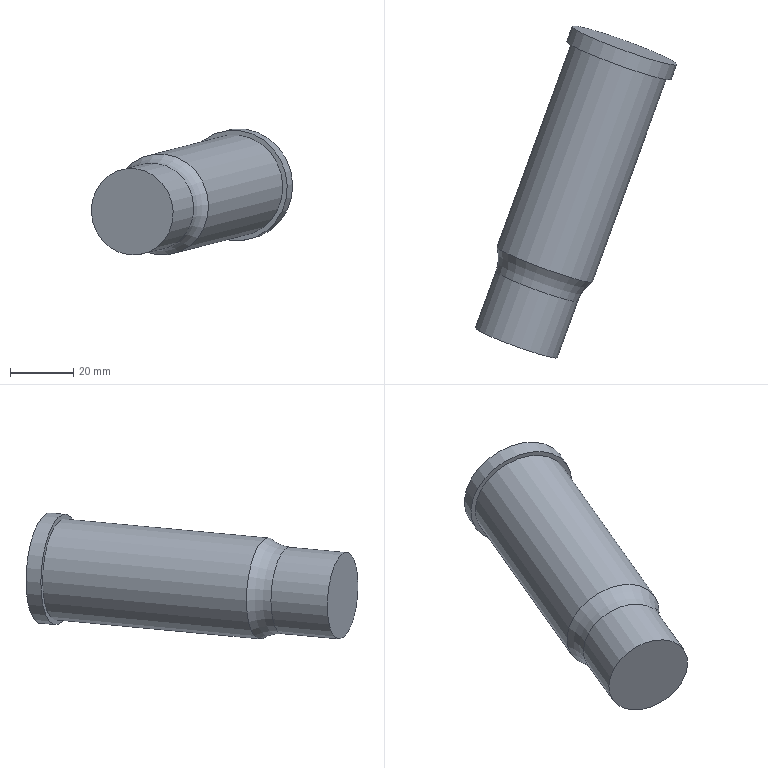Part | NX | features solid 2 | 1 solid | 7 faces | box 63.414 x 104.588 x 39.807 mm | volume 76067 mm3 | cylinder 3 | plane 3 | torus 1 | commonest cylinder face diameters 27.42 x1 32 x1 35 x1
STEP:
#1=CARTESIAN_POINT('',(-630.428,136.085,-11.472));
#2=VERTEX_POINT('',#1);
#3=CARTESIAN_POINT('',(-646.873,142.071,-11.472));
#4=DIRECTION('',(-0.3407,-0.9361,-0.08716));
#5=DIRECTION('',(0.9397,-0.342,0.));
#6=AXIS2_PLACEMENT_3D('',#3,#4,#5);
#7=CIRCLE('',#6,17.5);
#8=EDGE_CURVE('',#2,#2,#7,.T.);
#9=ORIENTED_EDGE('',*,*,#8,.F.);
#10=EDGE_LOOP('',(#9));
#11=FACE_BOUND('',#10,.T.);
#12=CARTESIAN_POINT('',(-628.725,140.766,-11.037));
#13=VERTEX_POINT('',#12);
#14=CARTESIAN_POINT('',(-645.169,146.751,-11.037));
#15=DIRECTION('',(-0.3407,-0.9361,-0.08716));
#16=DIRECTION('',(0.9397,-0.342,0.));
#17=AXIS2_PLACEMENT_3D('',#14,#15,#16);
#18=CIRCLE('',#17,17.5);
#19=EDGE_CURVE('',#13,#13,#18,.T.);
#20=ORIENTED_EDGE('',*,*,#19,.T.);
#21=EDGE_LOOP('',(#20));
#22=FACE_BOUND('',#21,.T.);
#23=CARTESIAN_POINT('',(-653.687,123.348,-13.216));
#24=DIRECTION('',(0.3407,0.9361,0.08716));
#25=DIRECTION('',(-0.9397,0.342,0.));
#26=AXIS2_PLACEMENT_3D('',#23,#24,#25);
#27=CYLINDRICAL_SURFACE('',#26,17.5);
#28=ADVANCED_FACE('',(#11,#22),#27,.T.);
#29=CARTESIAN_POINT('',(-631.838,136.598,-11.472));
#30=VERTEX_POINT('',#29);
#31=CARTESIAN_POINT('',(-646.873,142.071,-11.472));
#32=DIRECTION('',(-0.3407,-0.9361,-0.08716));
#33=DIRECTION('',(0.9397,-0.342,0.));
#34=AXIS2_PLACEMENT_3D('',#31,#32,#33);
#35=CIRCLE('',#34,16.);
#36=EDGE_CURVE('',#30,#30,#35,.T.);
#37=ORIENTED_EDGE('',*,*,#36,.F.);
#38=EDGE_LOOP('',(#37));
#39=FACE_BOUND('',#38,.T.);
#40=ORIENTED_EDGE('',*,*,#8,.T.);
#41=EDGE_LOOP('',(#40));
#42=FACE_BOUND('',#41,.T.);
#43=CARTESIAN_POINT('',(-646.873,142.071,-11.472));
#44=DIRECTION('',(-0.3407,-0.9361,-0.08716));
#45=DIRECTION('',(0.9397,-0.342,0.));
#46=AXIS2_PLACEMENT_3D('',#43,#44,#45);
#47=PLANE('',#46);
#48=ADVANCED_FACE('',(#39,#42),#47,.T.);
#49=ORIENTED_EDGE('',*,*,#19,.F.);
#50=EDGE_LOOP('',(#49));
#51=FACE_BOUND('',#50,.T.);
#52=CARTESIAN_POINT('',(-645.169,146.751,-11.037));
#53=DIRECTION('',(-0.3407,-0.9361,-0.08716));
#54=DIRECTION('',(0.9397,-0.342,0.));
#55=AXIS2_PLACEMENT_3D('',#52,#53,#54);
#56=PLANE('',#55);
#57=ADVANCED_FACE('',(#51),#56,.F.);
#58=ORIENTED_EDGE('',*,*,#36,.T.);
#59=EDGE_LOOP('',(#58));
#60=FACE_BOUND('',#59,.T.);
#61=CARTESIAN_POINT('',(-655.222,72.351,-17.454));
#62=VERTEX_POINT('',#61);
#63=CARTESIAN_POINT('',(-670.257,77.824,-17.454));
#64=DIRECTION('',(-0.3407,-0.9361,-0.08716));
#65=DIRECTION('',(0.9397,-0.342,0.));
#66=AXIS2_PLACEMENT_3D('',#63,#64,#65);
#67=CIRCLE('',#66,16.);
#68=EDGE_CURVE('',#62,#62,#67,.T.);
#69=ORIENTED_EDGE('',*,*,#68,.F.);
#70=EDGE_LOOP('',(#69));
#71=FACE_BOUND('',#70,.T.);
#72=CARTESIAN_POINT('',(-653.687,123.348,-13.216));
#73=DIRECTION('',(-0.3407,-0.9361,-0.08716));
#74=DIRECTION('',(0.9397,-0.342,0.));
#75=AXIS2_PLACEMENT_3D('',#72,#73,#74);
#76=CYLINDRICAL_SURFACE('',#75,16.);
#77=ADVANCED_FACE('',(#60,#71),#76,.T.);
#78=CARTESIAN_POINT('',(-685.651,75.615,-18.096));
#79=VERTEX_POINT('',#78);
#80=CARTESIAN_POINT('',(-672.767,70.926,-18.096));
#81=DIRECTION('',(0.3407,0.9361,0.08716));
#82=DIRECTION('',(-0.9397,0.342,0.));
#83=AXIS2_PLACEMENT_3D('',#80,#81,#82);
#84=CIRCLE('',#83,13.71);
#85=EDGE_CURVE('',#79,#79,#84,.F.);
#86=ORIENTED_EDGE('',*,*,#85,.T.);
#87=EDGE_LOOP('',(#86));
#88=FACE_BOUND('',#87,.T.);
#89=CARTESIAN_POINT('',(-666.358,48.451,-19.752));
#90=VERTEX_POINT('',#89);
#91=CARTESIAN_POINT('',(-679.241,53.14,-19.752));
#92=DIRECTION('',(-0.3407,-0.9361,-0.08716));
#93=DIRECTION('',(0.9397,-0.342,0.));
#94=AXIS2_PLACEMENT_3D('',#91,#92,#93);
#95=CIRCLE('',#94,13.71);
#96=EDGE_CURVE('',#90,#90,#95,.T.);
#97=ORIENTED_EDGE('',*,*,#96,.F.);
#98=EDGE_LOOP('',(#97));
#99=FACE_BOUND('',#98,.T.);
#100=CARTESIAN_POINT('',(-679.241,53.14,-19.752));
#101=DIRECTION('',(0.3407,0.9361,0.08716));
#102=DIRECTION('',(-0.9397,0.342,0.));
#103=AXIS2_PLACEMENT_3D('',#100,#101,#102);
#104=CYLINDRICAL_SURFACE('',#103,13.71);
#105=ADVANCED_FACE('',(#88,#99),#104,.T.);
#106=ORIENTED_EDGE('',*,*,#96,.T.);
#107=EDGE_LOOP('',(#106));
#108=FACE_BOUND('',#107,.T.);
#109=CARTESIAN_POINT('',(-679.241,53.14,-19.752));
#110=DIRECTION('',(-0.3407,-0.9361,-0.08716));
#111=DIRECTION('',(0.9397,-0.342,0.));
#112=AXIS2_PLACEMENT_3D('',#109,#110,#111);
#113=PLANE('',#112);
#114=ADVANCED_FACE('',(#108),#113,.T.);
#115=ORIENTED_EDGE('',*,*,#68,.T.);
#116=EDGE_LOOP('',(#115));
#117=FACE_BOUND('',#116,.T.);
#118=ORIENTED_EDGE('',*,*,#85,.F.);
#119=EDGE_LOOP('',(#118));
#120=FACE_BOUND('',#119,.T.);
#121=CARTESIAN_POINT('',(-672.767,70.926,-18.096));
#122=DIRECTION('',(0.3407,0.9361,0.08716));
#123=DIRECTION('',(-0.9397,0.342,0.));
#124=AXIS2_PLACEMENT_3D('',#121,#122,#123);
#125=TOROIDAL_SURFACE('',#124,26.71,13.);
#126=ADVANCED_FACE('',(#117,#120),#125,.F.);
#127=CLOSED_SHELL('',(#28,#48,#57,#77,#105,#114,#126));
#128=MANIFOLD_SOLID_BREP('',#127);
#129=(LENGTH_UNIT()NAMED_UNIT(*)SI_UNIT(.MILLI.,.METRE.));
#130=UNCERTAINTY_MEASURE_WITH_UNIT(LENGTH_MEASURE(0.00001),#129,'','');
#131=(NAMED_UNIT(*)PLANE_ANGLE_UNIT()SI_UNIT($,.RADIAN.));
#132=(NAMED_UNIT(*)SI_UNIT($,.STERADIAN.)SOLID_ANGLE_UNIT());
#133=(GEOMETRIC_REPRESENTATION_CONTEXT(3)GLOBAL_UNCERTAINTY_ASSIGNED_CONTEXT((#130))GLOBAL_UNIT_ASSIGNED_CONTEXT((#129,#131,#132))REPRESENTATION_CONTEXT('',''));
#134=ADVANCED_BREP_SHAPE_REPRESENTATION('',(#128),#133);